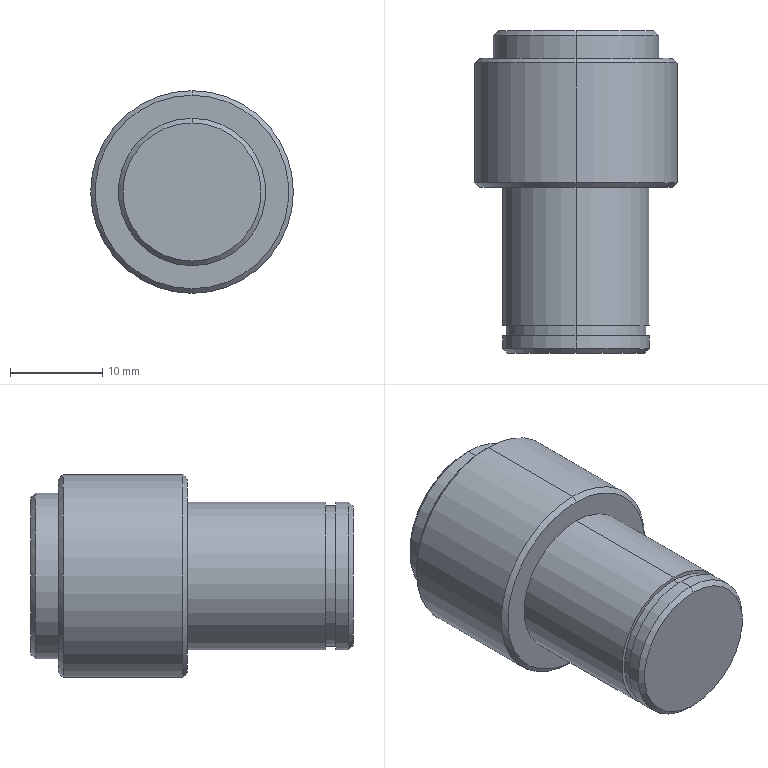Part | STEP file | 02-Support shaft 4 | 1 solid | 24 faces | box 22 x 35 x 22 mm | volume 9653 mm3 | cylinder 10 | cone 8 | plane 6 | commonest cylinder face diameters 16 x4 15.2 x2 18 x2 22 x2
STEP:
#1=CARTESIAN_POINT('',(0.,0.,0.));
#2=DIRECTION('',(0.,0.,1.));
#3=DIRECTION('',(1.,0.,0.));
#4=AXIS2_PLACEMENT_3D('',#1,#2,#3);
#5=CARTESIAN_POINT('',(0.,0.,8.5));
#6=VERTEX_POINT('',#5);
#7=CARTESIAN_POINT('',(0.,0.,-8.5));
#8=VERTEX_POINT('',#7);
#9=CARTESIAN_POINT('',(0.,0.,0.));
#10=DIRECTION('',(0.,1.,0.));
#11=DIRECTION('',(0.,0.,1.));
#12=AXIS2_PLACEMENT_3D('',#9,#10,#11);
#13=CIRCLE('',#12,8.5);
#14=CARTESIAN_POINT('',(0.,0.,0.));
#15=DIRECTION('',(0.,-1.,0.));
#16=DIRECTION('',(0.,0.,-1.));
#17=AXIS2_PLACEMENT_3D('',#14,#15,#16);
#18=CONICAL_SURFACE('',#17,8.5,0.7854);
#19=CARTESIAN_POINT('',(3.142,0.));
#20=DIRECTION('',(-1.,0.));
#21=VECTOR('',#20,1.);
#22=LINE('',#19,#21);
#23=(GEOMETRIC_REPRESENTATION_CONTEXT(2)PARAMETRIC_REPRESENTATION_CONTEXT()REPRESENTATION_CONTEXT('',''));
#24=DEFINITIONAL_REPRESENTATION('',(#22),#23);
#25=PCURVE('',#18,#24);
#26=CARTESIAN_POINT('',(0.,0.,0.));
#27=DIRECTION('',(0.,1.,0.));
#28=DIRECTION('',(0.,0.,1.));
#29=AXIS2_PLACEMENT_3D('',#26,#27,#28);
#30=PLANE('',#29);
#31=CARTESIAN_POINT('',(0.,0.));
#32=DIRECTION('',(1.,0.));
#33=AXIS2_PLACEMENT_2D('',#31,#32);
#34=CIRCLE('',#33,8.5);
#35=(GEOMETRIC_REPRESENTATION_CONTEXT(2)PARAMETRIC_REPRESENTATION_CONTEXT()REPRESENTATION_CONTEXT('',''));
#36=DEFINITIONAL_REPRESENTATION('',(#34),#35);
#37=PCURVE('',#30,#36);
#38=SURFACE_CURVE('',#13,(#25,#37),.PCURVE_S1.);
#39=EDGE_CURVE('',#6,#8,#38,.T.);
#40=ORIENTED_EDGE('',*,*,#39,.F.);
#41=CARTESIAN_POINT('',(0.,-0.5,9.));
#42=VERTEX_POINT('',#41);
#43=CARTESIAN_POINT('',(0.,0.,8.5));
#44=DIRECTION('',(0.,-0.7071,0.7071));
#45=VECTOR('',#44,1.);
#46=LINE('',#43,#45);
#47=CARTESIAN_POINT('',(3.142,0.));
#48=DIRECTION('',(0.,1.));
#49=VECTOR('',#48,1.);
#50=LINE('',#47,#49);
#51=(GEOMETRIC_REPRESENTATION_CONTEXT(2)PARAMETRIC_REPRESENTATION_CONTEXT()REPRESENTATION_CONTEXT('',''));
#52=DEFINITIONAL_REPRESENTATION('',(#50),#51);
#53=PCURVE('',#18,#52);
#54=CARTESIAN_POINT('',(0.,0.,0.));
#55=DIRECTION('',(0.,-1.,0.));
#56=DIRECTION('',(0.,0.,-1.));
#57=AXIS2_PLACEMENT_3D('',#54,#55,#56);
#58=CONICAL_SURFACE('',#57,8.5,0.7854);
#59=CARTESIAN_POINT('',(3.142,0.));
#60=DIRECTION('',(0.,1.));
#61=VECTOR('',#60,1.);
#62=LINE('',#59,#61);
#63=(GEOMETRIC_REPRESENTATION_CONTEXT(2)PARAMETRIC_REPRESENTATION_CONTEXT()REPRESENTATION_CONTEXT('',''));
#64=DEFINITIONAL_REPRESENTATION('',(#62),#63);
#65=PCURVE('',#58,#64);
#66=SURFACE_CURVE('',#46,(#53,#65),.PCURVE_S1.);
#67=EDGE_CURVE('',#6,#42,#66,.T.);
#68=ORIENTED_EDGE('',*,*,#67,.T.);
#69=CARTESIAN_POINT('',(0.,-0.5,-9.));
#70=VERTEX_POINT('',#69);
#71=CARTESIAN_POINT('',(0.,-0.5,0.));
#72=DIRECTION('',(0.,-1.,0.));
#73=DIRECTION('',(0.,0.,1.));
#74=AXIS2_PLACEMENT_3D('',#71,#72,#73);
#75=CIRCLE('',#74,9.);
#76=CARTESIAN_POINT('',(-3.142,0.5));
#77=DIRECTION('',(1.,0.));
#78=VECTOR('',#77,1.);
#79=LINE('',#76,#78);
#80=(GEOMETRIC_REPRESENTATION_CONTEXT(2)PARAMETRIC_REPRESENTATION_CONTEXT()REPRESENTATION_CONTEXT('',''));
#81=DEFINITIONAL_REPRESENTATION('',(#79),#80);
#82=PCURVE('',#18,#81);
#83=CARTESIAN_POINT('',(0.,0.,0.));
#84=DIRECTION('',(0.,1.,0.));
#85=DIRECTION('',(0.,0.,1.));
#86=AXIS2_PLACEMENT_3D('',#83,#84,#85);
#87=CYLINDRICAL_SURFACE('',#86,9.);
#88=CARTESIAN_POINT('',(6.283,-0.5));
#89=DIRECTION('',(-1.,0.));
#90=VECTOR('',#89,1.);
#91=LINE('',#88,#90);
#92=(GEOMETRIC_REPRESENTATION_CONTEXT(2)PARAMETRIC_REPRESENTATION_CONTEXT()REPRESENTATION_CONTEXT('',''));
#93=DEFINITIONAL_REPRESENTATION('',(#91),#92);
#94=PCURVE('',#87,#93);
#95=SURFACE_CURVE('',#75,(#82,#94),.PCURVE_S1.);
#96=EDGE_CURVE('',#70,#42,#95,.T.);
#97=ORIENTED_EDGE('',*,*,#96,.F.);
#98=CARTESIAN_POINT('',(0.,0.,-8.5));
#99=DIRECTION('',(0.,-0.7071,-0.7071));
#100=VECTOR('',#99,1.);
#101=LINE('',#98,#100);
#102=CARTESIAN_POINT('',(0.,0.));
#103=DIRECTION('',(0.,1.));
#104=VECTOR('',#103,1.);
#105=LINE('',#102,#104);
#106=(GEOMETRIC_REPRESENTATION_CONTEXT(2)PARAMETRIC_REPRESENTATION_CONTEXT()REPRESENTATION_CONTEXT('',''));
#107=DEFINITIONAL_REPRESENTATION('',(#105),#106);
#108=PCURVE('',#18,#107);
#109=CARTESIAN_POINT('',(6.283,0.));
#110=DIRECTION('',(0.,1.));
#111=VECTOR('',#110,1.);
#112=LINE('',#109,#111);
#113=(GEOMETRIC_REPRESENTATION_CONTEXT(2)PARAMETRIC_REPRESENTATION_CONTEXT()REPRESENTATION_CONTEXT('',''));
#114=DEFINITIONAL_REPRESENTATION('',(#112),#113);
#115=PCURVE('',#58,#114);
#116=SURFACE_CURVE('',#101,(#108,#115),.PCURVE_S1.);
#117=EDGE_CURVE('',#8,#70,#116,.T.);
#118=ORIENTED_EDGE('',*,*,#117,.F.);
#119=EDGE_LOOP('',(#40,#68,#97,#118));
#120=FACE_BOUND('',#119,.T.);
#121=ADVANCED_FACE('',(#120),#18,.T.);
#122=CARTESIAN_POINT('',(0.,-3.,10.5));
#123=VERTEX_POINT('',#122);
#124=CARTESIAN_POINT('',(0.,-3.,-10.5));
#125=VERTEX_POINT('',#124);
#126=CARTESIAN_POINT('',(0.,-3.,0.));
#127=DIRECTION('',(0.,1.,0.));
#128=DIRECTION('',(0.,0.,1.));
#129=AXIS2_PLACEMENT_3D('',#126,#127,#128);
#130=CIRCLE('',#129,10.5);
#131=CARTESIAN_POINT('',(0.,-3.,0.));
#132=DIRECTION('',(0.,-1.,0.));
#133=DIRECTION('',(0.,0.,-1.));
#134=AXIS2_PLACEMENT_3D('',#131,#132,#133);
#135=CONICAL_SURFACE('',#134,10.5,0.7854);
#136=CARTESIAN_POINT('',(3.142,0.));
#137=DIRECTION('',(-1.,0.));
#138=VECTOR('',#137,1.);
#139=LINE('',#136,#138);
#140=(GEOMETRIC_REPRESENTATION_CONTEXT(2)PARAMETRIC_REPRESENTATION_CONTEXT()REPRESENTATION_CONTEXT('',''));
#141=DEFINITIONAL_REPRESENTATION('',(#139),#140);
#142=PCURVE('',#135,#141);
#143=CARTESIAN_POINT('',(-9.,-3.,0.));
#144=DIRECTION('',(0.,1.,0.));
#145=DIRECTION('',(0.,0.,1.));
#146=AXIS2_PLACEMENT_3D('',#143,#144,#145);
#147=PLANE('',#146);
#148=CARTESIAN_POINT('',(0.,9.));
#149=DIRECTION('',(1.,0.));
#150=AXIS2_PLACEMENT_2D('',#148,#149);
#151=CIRCLE('',#150,10.5);
#152=(GEOMETRIC_REPRESENTATION_CONTEXT(2)PARAMETRIC_REPRESENTATION_CONTEXT()REPRESENTATION_CONTEXT('',''));
#153=DEFINITIONAL_REPRESENTATION('',(#151),#152);
#154=PCURVE('',#147,#153);
#155=SURFACE_CURVE('',#130,(#142,#154),.PCURVE_S1.);
#156=EDGE_CURVE('',#123,#125,#155,.T.);
#157=ORIENTED_EDGE('',*,*,#156,.F.);
#158=CARTESIAN_POINT('',(0.,-3.5,11.));
#159=VERTEX_POINT('',#158);
#160=CARTESIAN_POINT('',(0.,-3.,10.5));
#161=DIRECTION('',(0.,-0.7071,0.7071));
#162=VECTOR('',#161,1.);
#163=LINE('',#160,#162);
#164=CARTESIAN_POINT('',(3.142,0.));
#165=DIRECTION('',(0.,1.));
#166=VECTOR('',#165,1.);
#167=LINE('',#164,#166);
#168=(GEOMETRIC_REPRESENTATION_CONTEXT(2)PARAMETRIC_REPRESENTATION_CONTEXT()REPRESENTATION_CONTEXT('',''));
#169=DEFINITIONAL_REPRESENTATION('',(#167),#168);
#170=PCURVE('',#135,#169);
#171=CARTESIAN_POINT('',(0.,-3.,0.));
#172=DIRECTION('',(0.,-1.,0.));
#173=DIRECTION('',(0.,0.,-1.));
#174=AXIS2_PLACEMENT_3D('',#171,#172,#173);
#175=CONICAL_SURFACE('',#174,10.5,0.7854);
#176=CARTESIAN_POINT('',(3.142,0.));
#177=DIRECTION('',(0.,1.));
#178=VECTOR('',#177,1.);
#179=LINE('',#176,#178);
#180=(GEOMETRIC_REPRESENTATION_CONTEXT(2)PARAMETRIC_REPRESENTATION_CONTEXT()REPRESENTATION_CONTEXT('',''));
#181=DEFINITIONAL_REPRESENTATION('',(#179),#180);
#182=PCURVE('',#175,#181);
#183=SURFACE_CURVE('',#163,(#170,#182),.PCURVE_S1.);
#184=EDGE_CURVE('',#123,#159,#183,.T.);
#185=ORIENTED_EDGE('',*,*,#184,.T.);
#186=CARTESIAN_POINT('',(0.,-3.5,-11.));
#187=VERTEX_POINT('',#186);
#188=CARTESIAN_POINT('',(0.,-3.5,0.));
#189=DIRECTION('',(0.,-1.,0.));
#190=DIRECTION('',(0.,0.,1.));
#191=AXIS2_PLACEMENT_3D('',#188,#189,#190);
#192=CIRCLE('',#191,11.);
#193=CARTESIAN_POINT('',(-3.142,0.5));
#194=DIRECTION('',(1.,0.));
#195=VECTOR('',#194,1.);
#196=LINE('',#193,#195);
#197=(GEOMETRIC_REPRESENTATION_CONTEXT(2)PARAMETRIC_REPRESENTATION_CONTEXT()REPRESENTATION_CONTEXT('',''));
#198=DEFINITIONAL_REPRESENTATION('',(#196),#197);
#199=PCURVE('',#135,#198);
#200=CARTESIAN_POINT('',(0.,0.,0.));
#201=DIRECTION('',(0.,1.,0.));
#202=DIRECTION('',(0.,0.,1.));
#203=AXIS2_PLACEMENT_3D('',#200,#201,#202);
#204=CYLINDRICAL_SURFACE('',#203,11.);
#205=CARTESIAN_POINT('',(6.283,-3.5));
#206=DIRECTION('',(-1.,0.));
#207=VECTOR('',#206,1.);
#208=LINE('',#205,#207);
#209=(GEOMETRIC_REPRESENTATION_CONTEXT(2)PARAMETRIC_REPRESENTATION_CONTEXT()REPRESENTATION_CONTEXT('',''));
#210=DEFINITIONAL_REPRESENTATION('',(#208),#209);
#211=PCURVE('',#204,#210);
#212=SURFACE_CURVE('',#192,(#199,#211),.PCURVE_S1.);
#213=EDGE_CURVE('',#187,#159,#212,.T.);
#214=ORIENTED_EDGE('',*,*,#213,.F.);
#215=CARTESIAN_POINT('',(0.,-3.,-10.5));
#216=DIRECTION('',(0.,-0.7071,-0.7071));
#217=VECTOR('',#216,1.);
#218=LINE('',#215,#217);
#219=CARTESIAN_POINT('',(0.,0.));
#220=DIRECTION('',(0.,1.));
#221=VECTOR('',#220,1.);
#222=LINE('',#219,#221);
#223=(GEOMETRIC_REPRESENTATION_CONTEXT(2)PARAMETRIC_REPRESENTATION_CONTEXT()REPRESENTATION_CONTEXT('',''));
#224=DEFINITIONAL_REPRESENTATION('',(#222),#223);
#225=PCURVE('',#135,#224);
#226=CARTESIAN_POINT('',(6.283,0.));
#227=DIRECTION('',(0.,1.));
#228=VECTOR('',#227,1.);
#229=LINE('',#226,#228);
#230=(GEOMETRIC_REPRESENTATION_CONTEXT(2)PARAMETRIC_REPRESENTATION_CONTEXT()REPRESENTATION_CONTEXT('',''));
#231=DEFINITIONAL_REPRESENTATION('',(#229),#230);
#232=PCURVE('',#175,#231);
#233=SURFACE_CURVE('',#218,(#225,#232),.PCURVE_S1.);
#234=EDGE_CURVE('',#125,#187,#233,.T.);
#235=ORIENTED_EDGE('',*,*,#234,.F.);
#236=EDGE_LOOP('',(#157,#185,#214,#235));
#237=FACE_BOUND('',#236,.T.);
#238=ADVANCED_FACE('',(#237),#135,.T.);
#239=CARTESIAN_POINT('',(0.,-17.,-10.5));
#240=VERTEX_POINT('',#239);
#241=CARTESIAN_POINT('',(0.,-17.,10.5));
#242=VERTEX_POINT('',#241);
#243=CARTESIAN_POINT('',(0.,-17.,0.));
#244=DIRECTION('',(0.,-1.,0.));
#245=DIRECTION('',(0.,0.,-1.));
#246=AXIS2_PLACEMENT_3D('',#243,#244,#245);
#247=CIRCLE('',#246,10.5);
#248=CARTESIAN_POINT('',(0.,-16.5,0.));
#249=DIRECTION('',(0.,1.,0.));
#250=DIRECTION('',(0.,0.,1.));
#251=AXIS2_PLACEMENT_3D('',#248,#249,#250);
#252=CONICAL_SURFACE('',#251,11.,0.7854);
#253=CARTESIAN_POINT('',(3.142,-0.5));
#254=DIRECTION('',(-1.,0.));
#255=VECTOR('',#254,1.);
#256=LINE('',#253,#255);
#257=(GEOMETRIC_REPRESENTATION_CONTEXT(2)PARAMETRIC_REPRESENTATION_CONTEXT()REPRESENTATION_CONTEXT('',''));
#258=DEFINITIONAL_REPRESENTATION('',(#256),#257);
#259=PCURVE('',#252,#258);
#260=CARTESIAN_POINT('',(-11.,-17.,0.));
#261=DIRECTION('',(0.,-1.,0.));
#262=DIRECTION('',(0.,0.,-1.));
#263=AXIS2_PLACEMENT_3D('',#260,#261,#262);
#264=PLANE('',#263);
#265=CARTESIAN_POINT('',(0.,11.));
#266=DIRECTION('',(1.,0.));
#267=AXIS2_PLACEMENT_2D('',#265,#266);
#268=CIRCLE('',#267,10.5);
#269=(GEOMETRIC_REPRESENTATION_CONTEXT(2)PARAMETRIC_REPRESENTATION_CONTEXT()REPRESENTATION_CONTEXT('',''));
#270=DEFINITIONAL_REPRESENTATION('',(#268),#269);
#271=PCURVE('',#264,#270);
#272=SURFACE_CURVE('',#247,(#259,#271),.PCURVE_S1.);
#273=EDGE_CURVE('',#240,#242,#272,.T.);
#274=ORIENTED_EDGE('',*,*,#273,.F.);
#275=CARTESIAN_POINT('',(0.,-16.5,-11.));
#276=VERTEX_POINT('',#275);
#277=CARTESIAN_POINT('',(0.,-16.5,-11.));
#278=DIRECTION('',(0.,0.7071,-0.7071));
#279=VECTOR('',#278,1.);
#280=LINE('',#277,#279);
#281=CARTESIAN_POINT('',(3.142,0.));
#282=DIRECTION('',(0.,1.));
#283=VECTOR('',#282,1.);
#284=LINE('',#281,#283);
#285=(GEOMETRIC_REPRESENTATION_CONTEXT(2)PARAMETRIC_REPRESENTATION_CONTEXT()REPRESENTATION_CONTEXT('',''));
#286=DEFINITIONAL_REPRESENTATION('',(#284),#285);
#287=PCURVE('',#252,#286);
#288=CARTESIAN_POINT('',(0.,-16.5,0.));
#289=DIRECTION('',(0.,1.,0.));
#290=DIRECTION('',(0.,0.,1.));
#291=AXIS2_PLACEMENT_3D('',#288,#289,#290);
#292=CONICAL_SURFACE('',#291,11.,0.7854);
#293=CARTESIAN_POINT('',(3.142,0.));
#294=DIRECTION('',(0.,1.));
#295=VECTOR('',#294,1.);
#296=LINE('',#293,#295);
#297=(GEOMETRIC_REPRESENTATION_CONTEXT(2)PARAMETRIC_REPRESENTATION_CONTEXT()REPRESENTATION_CONTEXT('',''));
#298=DEFINITIONAL_REPRESENTATION('',(#296),#297);
#299=PCURVE('',#292,#298);
#300=SURFACE_CURVE('',#280,(#287,#299),.PCURVE_S1.);
#301=EDGE_CURVE('',#240,#276,#300,.T.);
#302=ORIENTED_EDGE('',*,*,#301,.T.);
#303=CARTESIAN_POINT('',(0.,-16.5,11.));
#304=VERTEX_POINT('',#303);
#305=CARTESIAN_POINT('',(0.,-16.5,0.));
#306=DIRECTION('',(0.,1.,0.));
#307=DIRECTION('',(0.,0.,-1.));
#308=AXIS2_PLACEMENT_3D('',#305,#306,#307);
#309=CIRCLE('',#308,11.);
#310=CARTESIAN_POINT('',(-3.142,0.));
#311=DIRECTION('',(1.,0.));
#312=VECTOR('',#311,1.);
#313=LINE('',#310,#312);
#314=(GEOMETRIC_REPRESENTATION_CONTEXT(2)PARAMETRIC_REPRESENTATION_CONTEXT()REPRESENTATION_CONTEXT('',''));
#315=DEFINITIONAL_REPRESENTATION('',(#313),#314);
#316=PCURVE('',#252,#315);
#317=CARTESIAN_POINT('',(-3.142,-16.5));
#318=DIRECTION('',(1.,0.));
#319=VECTOR('',#318,1.);
#320=LINE('',#317,#319);
#321=(GEOMETRIC_REPRESENTATION_CONTEXT(2)PARAMETRIC_REPRESENTATION_CONTEXT()REPRESENTATION_CONTEXT('',''));
#322=DEFINITIONAL_REPRESENTATION('',(#320),#321);
#323=PCURVE('',#204,#322);
#324=SURFACE_CURVE('',#309,(#316,#323),.PCURVE_S1.);
#325=EDGE_CURVE('',#304,#276,#324,.T.);
#326=ORIENTED_EDGE('',*,*,#325,.F.);
#327=CARTESIAN_POINT('',(0.,-16.5,11.));
#328=DIRECTION('',(0.,0.7071,0.7071));
#329=VECTOR('',#328,1.);
#330=LINE('',#327,#329);
#331=CARTESIAN_POINT('',(0.,0.));
#332=DIRECTION('',(0.,1.));
#333=VECTOR('',#332,1.);
#334=LINE('',#331,#333);
#335=(GEOMETRIC_REPRESENTATION_CONTEXT(2)PARAMETRIC_REPRESENTATION_CONTEXT()REPRESENTATION_CONTEXT('',''));
#336=DEFINITIONAL_REPRESENTATION('',(#334),#335);
#337=PCURVE('',#252,#336);
#338=CARTESIAN_POINT('',(6.283,0.));
#339=DIRECTION('',(0.,1.));
#340=VECTOR('',#339,1.);
#341=LINE('',#338,#340);
#342=(GEOMETRIC_REPRESENTATION_CONTEXT(2)PARAMETRIC_REPRESENTATION_CONTEXT()REPRESENTATION_CONTEXT('',''));
#343=DEFINITIONAL_REPRESENTATION('',(#341),#342);
#344=PCURVE('',#292,#343);
#345=SURFACE_CURVE('',#330,(#337,#344),.PCURVE_S1.);
#346=EDGE_CURVE('',#242,#304,#345,.T.);
#347=ORIENTED_EDGE('',*,*,#346,.F.);
#348=EDGE_LOOP('',(#274,#302,#326,#347));
#349=FACE_BOUND('',#348,.T.);
#350=ADVANCED_FACE('',(#349),#252,.T.);
#351=CARTESIAN_POINT('',(0.,-35.,-7.5));
#352=VERTEX_POINT('',#351);
#353=CARTESIAN_POINT('',(0.,-35.,7.5));
#354=VERTEX_POINT('',#353);
#355=CARTESIAN_POINT('',(0.,-35.,0.));
#356=DIRECTION('',(0.,-1.,0.));
#357=DIRECTION('',(0.,0.,-1.));
#358=AXIS2_PLACEMENT_3D('',#355,#356,#357);
#359=CIRCLE('',#358,7.5);
#360=CARTESIAN_POINT('',(0.,-34.5,0.));
#361=DIRECTION('',(0.,1.,0.));
#362=DIRECTION('',(0.,0.,1.));
#363=AXIS2_PLACEMENT_3D('',#360,#361,#362);
#364=CONICAL_SURFACE('',#363,8.,0.7854);
#365=CARTESIAN_POINT('',(3.142,-0.5));
#366=DIRECTION('',(-1.,0.));
#367=VECTOR('',#366,1.);
#368=LINE('',#365,#367);
#369=(GEOMETRIC_REPRESENTATION_CONTEXT(2)PARAMETRIC_REPRESENTATION_CONTEXT()REPRESENTATION_CONTEXT('',''));
#370=DEFINITIONAL_REPRESENTATION('',(#368),#369);
#371=PCURVE('',#364,#370);
#372=CARTESIAN_POINT('',(-8.,-35.,0.));
#373=DIRECTION('',(0.,-1.,0.));
#374=DIRECTION('',(0.,0.,-1.));
#375=AXIS2_PLACEMENT_3D('',#372,#373,#374);
#376=PLANE('',#375);
#377=CARTESIAN_POINT('',(0.,8.));
#378=DIRECTION('',(1.,0.));
#379=AXIS2_PLACEMENT_2D('',#377,#378);
#380=CIRCLE('',#379,7.5);
#381=(GEOMETRIC_REPRESENTATION_CONTEXT(2)PARAMETRIC_REPRESENTATION_CONTEXT()REPRESENTATION_CONTEXT('',''));
#382=DEFINITIONAL_REPRESENTATION('',(#380),#381);
#383=PCURVE('',#376,#382);
#384=SURFACE_CURVE('',#359,(#371,#383),.PCURVE_S1.);
#385=EDGE_CURVE('',#352,#354,#384,.T.);
#386=ORIENTED_EDGE('',*,*,#385,.F.);
#387=CARTESIAN_POINT('',(0.,-34.5,-8.));
#388=VERTEX_POINT('',#387);
#389=CARTESIAN_POINT('',(0.,-34.5,-8.));
#390=DIRECTION('',(0.,0.7071,-0.7071));
#391=VECTOR('',#390,1.);
#392=LINE('',#389,#391);
#393=CARTESIAN_POINT('',(3.142,0.));
#394=DIRECTION('',(0.,1.));
#395=VECTOR('',#394,1.);
#396=LINE('',#393,#395);
#397=(GEOMETRIC_REPRESENTATION_CONTEXT(2)PARAMETRIC_REPRESENTATION_CONTEXT()REPRESENTATION_CONTEXT('',''));
#398=DEFINITIONAL_REPRESENTATION('',(#396),#397);
#399=PCURVE('',#364,#398);
#400=CARTESIAN_POINT('',(0.,-34.5,0.));
#401=DIRECTION('',(0.,1.,0.));
#402=DIRECTION('',(0.,0.,1.));
#403=AXIS2_PLACEMENT_3D('',#400,#401,#402);
#404=CONICAL_SURFACE('',#403,8.,0.7854);
#405=CARTESIAN_POINT('',(3.142,0.));
#406=DIRECTION('',(0.,1.));
#407=VECTOR('',#406,1.);
#408=LINE('',#405,#407);
#409=(GEOMETRIC_REPRESENTATION_CONTEXT(2)PARAMETRIC_REPRESENTATION_CONTEXT()REPRESENTATION_CONTEXT('',''));
#410=DEFINITIONAL_REPRESENTATION('',(#408),#409);
#411=PCURVE('',#404,#410);
#412=SURFACE_CURVE('',#392,(#399,#411),.PCURVE_S1.);
#413=EDGE_CURVE('',#352,#388,#412,.T.);
#414=ORIENTED_EDGE('',*,*,#413,.T.);
#415=CARTESIAN_POINT('',(0.,-34.5,8.));
#416=VERTEX_POINT('',#415);
#417=CARTESIAN_POINT('',(0.,-34.5,0.));
#418=DIRECTION('',(0.,1.,0.));
#419=DIRECTION('',(0.,0.,-1.));
#420=AXIS2_PLACEMENT_3D('',#417,#418,#419);
#421=CIRCLE('',#420,8.);
#422=CARTESIAN_POINT('',(-3.142,0.));
#423=DIRECTION('',(1.,0.));
#424=VECTOR('',#423,1.);
#425=LINE('',#422,#424);
#426=(GEOMETRIC_REPRESENTATION_CONTEXT(2)PARAMETRIC_REPRESENTATION_CONTEXT()REPRESENTATION_CONTEXT('',''));
#427=DEFINITIONAL_REPRESENTATION('',(#425),#426);
#428=PCURVE('',#364,#427);
#429=CARTESIAN_POINT('',(0.,0.,0.));
#430=DIRECTION('',(0.,1.,0.));
#431=DIRECTION('',(0.,0.,1.));
#432=AXIS2_PLACEMENT_3D('',#429,#430,#431);
#433=CYLINDRICAL_SURFACE('',#432,8.);
#434=CARTESIAN_POINT('',(-3.142,-34.5));
#435=DIRECTION('',(1.,0.));
#436=VECTOR('',#435,1.);
#437=LINE('',#434,#436);
#438=(GEOMETRIC_REPRESENTATION_CONTEXT(2)PARAMETRIC_REPRESENTATION_CONTEXT()REPRESENTATION_CONTEXT('',''));
#439=DEFINITIONAL_REPRESENTATION('',(#437),#438);
#440=PCURVE('',#433,#439);
#441=SURFACE_CURVE('',#421,(#428,#440),.PCURVE_S1.);
#442=EDGE_CURVE('',#416,#388,#441,.T.);
#443=ORIENTED_EDGE('',*,*,#442,.F.);
#444=CARTESIAN_POINT('',(0.,-34.5,8.));
#445=DIRECTION('',(0.,0.7071,0.7071));
#446=VECTOR('',#445,1.);
#447=LINE('',#444,#446);
#448=CARTESIAN_POINT('',(0.,0.));
#449=DIRECTION('',(0.,1.));
#450=VECTOR('',#449,1.);
#451=LINE('',#448,#450);
#452=(GEOMETRIC_REPRESENTATION_CONTEXT(2)PARAMETRIC_REPRESENTATION_CONTEXT()REPRESENTATION_CONTEXT('',''));
#453=DEFINITIONAL_REPRESENTATION('',(#451),#452);
#454=PCURVE('',#364,#453);
#455=CARTESIAN_POINT('',(6.283,0.));
#456=DIRECTION('',(0.,1.));
#457=VECTOR('',#456,1.);
#458=LINE('',#455,#457);
#459=(GEOMETRIC_REPRESENTATION_CONTEXT(2)PARAMETRIC_REPRESENTATION_CONTEXT()REPRESENTATION_CONTEXT('',''));
#460=DEFINITIONAL_REPRESENTATION('',(#458),#459);
#461=PCURVE('',#404,#460);
#462=SURFACE_CURVE('',#447,(#454,#461),.PCURVE_S1.);
#463=EDGE_CURVE('',#354,#416,#462,.T.);
#464=ORIENTED_EDGE('',*,*,#463,.F.);
#465=EDGE_LOOP('',(#386,#414,#443,#464));
#466=FACE_BOUND('',#465,.T.);
#467=ADVANCED_FACE('',(#466),#364,.T.);
#468=ORIENTED_EDGE('',*,*,#442,.T.);
#469=CARTESIAN_POINT('',(0.,-33.1,-8.));
#470=VERTEX_POINT('',#469);
#471=CARTESIAN_POINT('',(0.,0.,-8.));
#472=DIRECTION('',(0.,1.,0.));
#473=VECTOR('',#472,1.);
#474=LINE('',#471,#473);
#475=CARTESIAN_POINT('',(3.142,0.));
#476=DIRECTION('',(0.,1.));
#477=VECTOR('',#476,1.);
#478=LINE('',#475,#477);
#479=(GEOMETRIC_REPRESENTATION_CONTEXT(2)PARAMETRIC_REPRESENTATION_CONTEXT()REPRESENTATION_CONTEXT('',''));
#480=DEFINITIONAL_REPRESENTATION('',(#478),#479);
#481=PCURVE('',#433,#480);
#482=CARTESIAN_POINT('',(0.,0.,0.));
#483=DIRECTION('',(0.,1.,0.));
#484=DIRECTION('',(0.,0.,1.));
#485=AXIS2_PLACEMENT_3D('',#482,#483,#484);
#486=CYLINDRICAL_SURFACE('',#485,8.);
#487=CARTESIAN_POINT('',(3.142,0.));
#488=DIRECTION('',(0.,1.));
#489=VECTOR('',#488,1.);
#490=LINE('',#487,#489);
#491=(GEOMETRIC_REPRESENTATION_CONTEXT(2)PARAMETRIC_REPRESENTATION_CONTEXT()REPRESENTATION_CONTEXT('',''));
#492=DEFINITIONAL_REPRESENTATION('',(#490),#491);
#493=PCURVE('',#486,#492);
#494=SURFACE_CURVE('',#474,(#481,#493),.PCURVE_S1.);
#495=EDGE_CURVE('',#388,#470,#494,.T.);
#496=ORIENTED_EDGE('',*,*,#495,.T.);
#497=CARTESIAN_POINT('',(0.,-33.1,8.));
#498=VERTEX_POINT('',#497);
#499=CARTESIAN_POINT('',(0.,-33.1,0.));
#500=DIRECTION('',(0.,1.,0.));
#501=DIRECTION('',(0.,0.,1.));
#502=AXIS2_PLACEMENT_3D('',#499,#500,#501);
#503=CIRCLE('',#502,8.);
#504=CARTESIAN_POINT('',(0.,-33.1));
#505=DIRECTION('',(1.,0.));
#506=VECTOR('',#505,1.);
#507=LINE('',#504,#506);
#508=(GEOMETRIC_REPRESENTATION_CONTEXT(2)PARAMETRIC_REPRESENTATION_CONTEXT()REPRESENTATION_CONTEXT('',''));
#509=DEFINITIONAL_REPRESENTATION('',(#507),#508);
#510=PCURVE('',#433,#509);
#511=CARTESIAN_POINT('',(-7.6,-33.1,0.));
#512=DIRECTION('',(0.,1.,0.));
#513=DIRECTION('',(0.,0.,1.));
#514=AXIS2_PLACEMENT_3D('',#511,#512,#513);
#515=PLANE('',#514);
#516=CARTESIAN_POINT('',(0.,7.6));
#517=DIRECTION('',(1.,0.));
#518=AXIS2_PLACEMENT_2D('',#516,#517);
#519=CIRCLE('',#518,8.);
#520=(GEOMETRIC_REPRESENTATION_CONTEXT(2)PARAMETRIC_REPRESENTATION_CONTEXT()REPRESENTATION_CONTEXT('',''));
#521=DEFINITIONAL_REPRESENTATION('',(#519),#520);
#522=PCURVE('',#515,#521);
#523=SURFACE_CURVE('',#503,(#510,#522),.PCURVE_S1.);
#524=EDGE_CURVE('',#498,#470,#523,.T.);
#525=ORIENTED_EDGE('',*,*,#524,.F.);
#526=CARTESIAN_POINT('',(0.,0.,8.));
#527=DIRECTION('',(0.,1.,0.));
#528=VECTOR('',#527,1.);
#529=LINE('',#526,#528);
#530=CARTESIAN_POINT('',(0.,0.));
#531=DIRECTION('',(0.,1.));
#532=VECTOR('',#531,1.);
#533=LINE('',#530,#532);
#534=(GEOMETRIC_REPRESENTATION_CONTEXT(2)PARAMETRIC_REPRESENTATION_CONTEXT()REPRESENTATION_CONTEXT('',''));
#535=DEFINITIONAL_REPRESENTATION('',(#533),#534);
#536=PCURVE('',#433,#535);
#537=CARTESIAN_POINT('',(6.283,0.));
#538=DIRECTION('',(0.,1.));
#539=VECTOR('',#538,1.);
#540=LINE('',#537,#539);
#541=(GEOMETRIC_REPRESENTATION_CONTEXT(2)PARAMETRIC_REPRESENTATION_CONTEXT()REPRESENTATION_CONTEXT('',''));
#542=DEFINITIONAL_REPRESENTATION('',(#540),#541);
#543=PCURVE('',#486,#542);
#544=SURFACE_CURVE('',#529,(#536,#543),.PCURVE_S1.);
#545=EDGE_CURVE('',#416,#498,#544,.T.);
#546=ORIENTED_EDGE('',*,*,#545,.F.);
#547=EDGE_LOOP('',(#468,#496,#525,#546));
#548=FACE_BOUND('',#547,.T.);
#549=ADVANCED_FACE('',(#548),#433,.T.);
#550=CARTESIAN_POINT('',(0.,-33.1,7.6));
#551=VERTEX_POINT('',#550);
#552=CARTESIAN_POINT('',(0.,-33.1,-7.6));
#553=VERTEX_POINT('',#552);
#554=CARTESIAN_POINT('',(0.,-33.1,0.));
#555=DIRECTION('',(0.,1.,0.));
#556=DIRECTION('',(0.,0.,1.));
#557=AXIS2_PLACEMENT_3D('',#554,#555,#556);
#558=CIRCLE('',#557,7.6);
#559=CARTESIAN_POINT('',(0.,0.,0.));
#560=DIRECTION('',(0.,1.,0.));
#561=DIRECTION('',(0.,0.,1.));
#562=AXIS2_PLACEMENT_3D('',#559,#560,#561);
#563=CYLINDRICAL_SURFACE('',#562,7.6);
#564=CARTESIAN_POINT('',(0.,-33.1));
#565=DIRECTION('',(1.,0.));
#566=VECTOR('',#565,1.);
#567=LINE('',#564,#566);
#568=(GEOMETRIC_REPRESENTATION_CONTEXT(2)PARAMETRIC_REPRESENTATION_CONTEXT()REPRESENTATION_CONTEXT('',''));
#569=DEFINITIONAL_REPRESENTATION('',(#567),#568);
#570=PCURVE('',#563,#569);
#571=CARTESIAN_POINT('',(0.,7.6));
#572=DIRECTION('',(1.,0.));
#573=AXIS2_PLACEMENT_2D('',#571,#572);
#574=CIRCLE('',#573,7.6);
#575=(GEOMETRIC_REPRESENTATION_CONTEXT(2)PARAMETRIC_REPRESENTATION_CONTEXT()REPRESENTATION_CONTEXT('',''));
#576=DEFINITIONAL_REPRESENTATION('',(#574),#575);
#577=PCURVE('',#515,#576);
#578=SURFACE_CURVE('',#558,(#570,#577),.PCURVE_S1.);
#579=EDGE_CURVE('',#551,#553,#578,.T.);
#580=ORIENTED_EDGE('',*,*,#579,.T.);
#581=CARTESIAN_POINT('',(0.,-32.,-7.6));
#582=VERTEX_POINT('',#581);
#583=CARTESIAN_POINT('',(0.,0.,-7.6));
#584=DIRECTION('',(0.,1.,0.));
#585=VECTOR('',#584,1.);
#586=LINE('',#583,#585);
#587=CARTESIAN_POINT('',(3.142,0.));
#588=DIRECTION('',(0.,1.));
#589=VECTOR('',#588,1.);
#590=LINE('',#587,#589);
#591=(GEOMETRIC_REPRESENTATION_CONTEXT(2)PARAMETRIC_REPRESENTATION_CONTEXT()REPRESENTATION_CONTEXT('',''));
#592=DEFINITIONAL_REPRESENTATION('',(#590),#591);
#593=PCURVE('',#563,#592);
#594=CARTESIAN_POINT('',(0.,0.,0.));
#595=DIRECTION('',(0.,1.,0.));
#596=DIRECTION('',(0.,0.,1.));
#597=AXIS2_PLACEMENT_3D('',#594,#595,#596);
#598=CYLINDRICAL_SURFACE('',#597,7.6);
#599=CARTESIAN_POINT('',(3.142,0.));
#600=DIRECTION('',(0.,1.));
#601=VECTOR('',#600,1.);
#602=LINE('',#599,#601);
#603=(GEOMETRIC_REPRESENTATION_CONTEXT(2)PARAMETRIC_REPRESENTATION_CONTEXT()REPRESENTATION_CONTEXT('',''));
#604=DEFINITIONAL_REPRESENTATION('',(#602),#603);
#605=PCURVE('',#598,#604);
#606=SURFACE_CURVE('',#586,(#593,#605),.PCURVE_S1.);
#607=EDGE_CURVE('',#553,#582,#606,.T.);
#608=ORIENTED_EDGE('',*,*,#607,.T.);
#609=CARTESIAN_POINT('',(0.,-32.,7.6));
#610=VERTEX_POINT('',#609);
#611=CARTESIAN_POINT('',(0.,-32.,0.));
#612=DIRECTION('',(0.,1.,0.));
#613=DIRECTION('',(0.,0.,1.));
#614=AXIS2_PLACEMENT_3D('',#611,#612,#613);
#615=CIRCLE('',#614,7.6);
#616=CARTESIAN_POINT('',(0.,-32.));
#617=DIRECTION('',(1.,0.));
#618=VECTOR('',#617,1.);
#619=LINE('',#616,#618);
#620=(GEOMETRIC_REPRESENTATION_CONTEXT(2)PARAMETRIC_REPRESENTATION_CONTEXT()REPRESENTATION_CONTEXT('',''));
#621=DEFINITIONAL_REPRESENTATION('',(#619),#620);
#622=PCURVE('',#563,#621);
#623=CARTESIAN_POINT('',(-8.,-32.,0.));
#624=DIRECTION('',(0.,-1.,0.));
#625=DIRECTION('',(0.,0.,-1.));
#626=AXIS2_PLACEMENT_3D('',#623,#624,#625);
#627=PLANE('',#626);
#628=CARTESIAN_POINT('',(-7.6,8.));
#629=CARTESIAN_POINT('',(-7.6,21.164));
#630=CARTESIAN_POINT('',(3.8,14.582));
#631=CARTESIAN_POINT('',(15.2,8.));
#632=CARTESIAN_POINT('',(3.8,1.418));
#633=CARTESIAN_POINT('',(-7.6,-5.164));
#634=CARTESIAN_POINT('',(-7.6,8.));
#635=(BOUNDED_CURVE()B_SPLINE_CURVE(2,(#628,#629,#630,#631,#632,#633,#634),.UNSPECIFIED.,.T.,.F.)B_SPLINE_CURVE_WITH_KNOTS((1,2,2,2,2,1),(-2.094,0.,2.094,4.189,6.283,8.378),.UNSPECIFIED.)CURVE()GEOMETRIC_REPRESENTATION_ITEM()RATIONAL_B_SPLINE_CURVE((1.,0.5,1.,0.5,1.,0.5,1.))REPRESENTATION_ITEM(''));
#636=(GEOMETRIC_REPRESENTATION_CONTEXT(2)PARAMETRIC_REPRESENTATION_CONTEXT()REPRESENTATION_CONTEXT('',''));
#637=DEFINITIONAL_REPRESENTATION('',(#635),#636);
#638=PCURVE('',#627,#637);
#639=SURFACE_CURVE('',#615,(#622,#638),.PCURVE_S1.);
#640=EDGE_CURVE('',#610,#582,#639,.T.);
#641=ORIENTED_EDGE('',*,*,#640,.F.);
#642=CARTESIAN_POINT('',(0.,0.,7.6));
#643=DIRECTION('',(0.,1.,0.));
#644=VECTOR('',#643,1.);
#645=LINE('',#642,#644);
#646=CARTESIAN_POINT('',(0.,0.));
#647=DIRECTION('',(0.,1.));
#648=VECTOR('',#647,1.);
#649=LINE('',#646,#648);
#650=(GEOMETRIC_REPRESENTATION_CONTEXT(2)PARAMETRIC_REPRESENTATION_CONTEXT()REPRESENTATION_CONTEXT('',''));
#651=DEFINITIONAL_REPRESENTATION('',(#649),#650);
#652=PCURVE('',#563,#651);
#653=CARTESIAN_POINT('',(6.283,0.));
#654=DIRECTION('',(0.,1.));
#655=VECTOR('',#654,1.);
#656=LINE('',#653,#655);
#657=(GEOMETRIC_REPRESENTATION_CONTEXT(2)PARAMETRIC_REPRESENTATION_CONTEXT()REPRESENTATION_CONTEXT('',''));
#658=DEFINITIONAL_REPRESENTATION('',(#656),#657);
#659=PCURVE('',#598,#658);
#660=SURFACE_CURVE('',#645,(#652,#659),.PCURVE_S1.);
#661=EDGE_CURVE('',#551,#610,#660,.T.);
#662=ORIENTED_EDGE('',*,*,#661,.F.);
#663=EDGE_LOOP('',(#580,#608,#641,#662));
#664=FACE_BOUND('',#663,.T.);
#665=ADVANCED_FACE('',(#664),#563,.T.);
#666=CARTESIAN_POINT('',(0.,-32.,8.));
#667=VERTEX_POINT('',#666);
#668=CARTESIAN_POINT('',(0.,-32.,-8.));
#669=VERTEX_POINT('',#668);
#670=CARTESIAN_POINT('',(0.,-32.,0.));
#671=DIRECTION('',(0.,1.,0.));
#672=DIRECTION('',(0.,0.,1.));
#673=AXIS2_PLACEMENT_3D('',#670,#671,#672);
#674=CIRCLE('',#673,8.);
#675=CARTESIAN_POINT('',(0.,0.,0.));
#676=DIRECTION('',(0.,1.,0.));
#677=DIRECTION('',(0.,0.,1.));
#678=AXIS2_PLACEMENT_3D('',#675,#676,#677);
#679=CYLINDRICAL_SURFACE('',#678,8.);
#680=CARTESIAN_POINT('',(0.,-32.));
#681=DIRECTION('',(1.,0.));
#682=VECTOR('',#681,1.);
#683=LINE('',#680,#682);
#684=(GEOMETRIC_REPRESENTATION_CONTEXT(2)PARAMETRIC_REPRESENTATION_CONTEXT()REPRESENTATION_CONTEXT('',''));
#685=DEFINITIONAL_REPRESENTATION('',(#683),#684);
#686=PCURVE('',#679,#685);
#687=CARTESIAN_POINT('',(-8.,8.));
#688=CARTESIAN_POINT('',(-8.,21.856));
#689=CARTESIAN_POINT('',(4.,14.928));
#690=CARTESIAN_POINT('',(16.,8.));
#691=CARTESIAN_POINT('',(4.,1.072));
#692=CARTESIAN_POINT('',(-8.,-5.856));
#693=CARTESIAN_POINT('',(-8.,8.));
#694=(BOUNDED_CURVE()B_SPLINE_CURVE(2,(#687,#688,#689,#690,#691,#692,#693),.UNSPECIFIED.,.T.,.F.)B_SPLINE_CURVE_WITH_KNOTS((1,2,2,2,2,1),(-2.094,0.,2.094,4.189,6.283,8.378),.UNSPECIFIED.)CURVE()GEOMETRIC_REPRESENTATION_ITEM()RATIONAL_B_SPLINE_CURVE((1.,0.5,1.,0.5,1.,0.5,1.))REPRESENTATION_ITEM(''));
#695=(GEOMETRIC_REPRESENTATION_CONTEXT(2)PARAMETRIC_REPRESENTATION_CONTEXT()REPRESENTATION_CONTEXT('',''));
#696=DEFINITIONAL_REPRESENTATION('',(#694),#695);
#697=PCURVE('',#627,#696);
#698=SURFACE_CURVE('',#674,(#686,#697),.PCURVE_S1.);
#699=EDGE_CURVE('',#667,#669,#698,.T.);
#700=ORIENTED_EDGE('',*,*,#699,.T.);
#701=CARTESIAN_POINT('',(0.,-17.,-8.));
#702=VERTEX_POINT('',#701);
#703=CARTESIAN_POINT('',(0.,0.,-8.));
#704=DIRECTION('',(0.,1.,0.));
#705=VECTOR('',#704,1.);
#706=LINE('',#703,#705);
#707=CARTESIAN_POINT('',(3.142,0.));
#708=DIRECTION('',(0.,1.));
#709=VECTOR('',#708,1.);
#710=LINE('',#707,#709);
#711=(GEOMETRIC_REPRESENTATION_CONTEXT(2)PARAMETRIC_REPRESENTATION_CONTEXT()REPRESENTATION_CONTEXT('',''));
#712=DEFINITIONAL_REPRESENTATION('',(#710),#711);
#713=PCURVE('',#679,#712);
#714=CARTESIAN_POINT('',(0.,0.,0.));
#715=DIRECTION('',(0.,1.,0.));
#716=DIRECTION('',(0.,0.,1.));
#717=AXIS2_PLACEMENT_3D('',#714,#715,#716);
#718=CYLINDRICAL_SURFACE('',#717,8.);
#719=CARTESIAN_POINT('',(3.142,0.));
#720=DIRECTION('',(0.,1.));
#721=VECTOR('',#720,1.);
#722=LINE('',#719,#721);
#723=(GEOMETRIC_REPRESENTATION_CONTEXT(2)PARAMETRIC_REPRESENTATION_CONTEXT()REPRESENTATION_CONTEXT('',''));
#724=DEFINITIONAL_REPRESENTATION('',(#722),#723);
#725=PCURVE('',#718,#724);
#726=SURFACE_CURVE('',#706,(#713,#725),.PCURVE_S1.);
#727=EDGE_CURVE('',#669,#702,#726,.T.);
#728=ORIENTED_EDGE('',*,*,#727,.T.);
#729=CARTESIAN_POINT('',(0.,-17.,8.));
#730=VERTEX_POINT('',#729);
#731=CARTESIAN_POINT('',(0.,-17.,0.));
#732=DIRECTION('',(0.,1.,0.));
#733=DIRECTION('',(0.,0.,1.));
#734=AXIS2_PLACEMENT_3D('',#731,#732,#733);
#735=CIRCLE('',#734,8.);
#736=CARTESIAN_POINT('',(0.,-17.));
#737=DIRECTION('',(1.,0.));
#738=VECTOR('',#737,1.);
#739=LINE('',#736,#738);
#740=(GEOMETRIC_REPRESENTATION_CONTEXT(2)PARAMETRIC_REPRESENTATION_CONTEXT()REPRESENTATION_CONTEXT('',''));
#741=DEFINITIONAL_REPRESENTATION('',(#739),#740);
#742=PCURVE('',#679,#741);
#743=CARTESIAN_POINT('',(-8.,11.));
#744=CARTESIAN_POINT('',(-8.,24.856));
#745=CARTESIAN_POINT('',(4.,17.928));
#746=CARTESIAN_POINT('',(16.,11.));
#747=CARTESIAN_POINT('',(4.,4.072));
#748=CARTESIAN_POINT('',(-8.,-2.856));
#749=CARTESIAN_POINT('',(-8.,11.));
#750=(BOUNDED_CURVE()B_SPLINE_CURVE(2,(#743,#744,#745,#746,#747,#748,#749),.UNSPECIFIED.,.T.,.F.)B_SPLINE_CURVE_WITH_KNOTS((1,2,2,2,2,1),(-2.094,0.,2.094,4.189,6.283,8.378),.UNSPECIFIED.)CURVE()GEOMETRIC_REPRESENTATION_ITEM()RATIONAL_B_SPLINE_CURVE((1.,0.5,1.,0.5,1.,0.5,1.))REPRESENTATION_ITEM(''));
#751=(GEOMETRIC_REPRESENTATION_CONTEXT(2)PARAMETRIC_REPRESENTATION_CONTEXT()REPRESENTATION_CONTEXT('',''));
#752=DEFINITIONAL_REPRESENTATION('',(#750),#751);
#753=PCURVE('',#264,#752);
#754=SURFACE_CURVE('',#735,(#742,#753),.PCURVE_S1.);
#755=EDGE_CURVE('',#730,#702,#754,.T.);
#756=ORIENTED_EDGE('',*,*,#755,.F.);
#757=CARTESIAN_POINT('',(0.,0.,8.));
#758=DIRECTION('',(0.,1.,0.));
#759=VECTOR('',#758,1.);
#760=LINE('',#757,#759);
#761=CARTESIAN_POINT('',(0.,0.));
#762=DIRECTION('',(0.,1.));
#763=VECTOR('',#762,1.);
#764=LINE('',#761,#763);
#765=(GEOMETRIC_REPRESENTATION_CONTEXT(2)PARAMETRIC_REPRESENTATION_CONTEXT()REPRESENTATION_CONTEXT('',''));
#766=DEFINITIONAL_REPRESENTATION('',(#764),#765);
#767=PCURVE('',#679,#766);
#768=CARTESIAN_POINT('',(6.283,0.));
#769=DIRECTION('',(0.,1.));
#770=VECTOR('',#769,1.);
#771=LINE('',#768,#770);
#772=(GEOMETRIC_REPRESENTATION_CONTEXT(2)PARAMETRIC_REPRESENTATION_CONTEXT()REPRESENTATION_CONTEXT('',''));
#773=DEFINITIONAL_REPRESENTATION('',(#771),#772);
#774=PCURVE('',#718,#773);
#775=SURFACE_CURVE('',#760,(#767,#774),.PCURVE_S1.);
#776=EDGE_CURVE('',#667,#730,#775,.T.);
#777=ORIENTED_EDGE('',*,*,#776,.F.);
#778=EDGE_LOOP('',(#700,#728,#756,#777));
#779=FACE_BOUND('',#778,.T.);
#780=ADVANCED_FACE('',(#779),#679,.T.);
#781=ORIENTED_EDGE('',*,*,#325,.T.);
#782=CARTESIAN_POINT('',(0.,0.,-11.));
#783=DIRECTION('',(0.,1.,0.));
#784=VECTOR('',#783,1.);
#785=LINE('',#782,#784);
#786=CARTESIAN_POINT('',(3.142,0.));
#787=DIRECTION('',(0.,1.));
#788=VECTOR('',#787,1.);
#789=LINE('',#786,#788);
#790=(GEOMETRIC_REPRESENTATION_CONTEXT(2)PARAMETRIC_REPRESENTATION_CONTEXT()REPRESENTATION_CONTEXT('',''));
#791=DEFINITIONAL_REPRESENTATION('',(#789),#790);
#792=PCURVE('',#204,#791);
#793=CARTESIAN_POINT('',(0.,0.,0.));
#794=DIRECTION('',(0.,1.,0.));
#795=DIRECTION('',(0.,0.,1.));
#796=AXIS2_PLACEMENT_3D('',#793,#794,#795);
#797=CYLINDRICAL_SURFACE('',#796,11.);
#798=CARTESIAN_POINT('',(3.142,0.));
#799=DIRECTION('',(0.,1.));
#800=VECTOR('',#799,1.);
#801=LINE('',#798,#800);
#802=(GEOMETRIC_REPRESENTATION_CONTEXT(2)PARAMETRIC_REPRESENTATION_CONTEXT()REPRESENTATION_CONTEXT('',''));
#803=DEFINITIONAL_REPRESENTATION('',(#801),#802);
#804=PCURVE('',#797,#803);
#805=SURFACE_CURVE('',#785,(#792,#804),.PCURVE_S1.);
#806=EDGE_CURVE('',#276,#187,#805,.T.);
#807=ORIENTED_EDGE('',*,*,#806,.T.);
#808=ORIENTED_EDGE('',*,*,#213,.T.);
#809=CARTESIAN_POINT('',(0.,0.,11.));
#810=DIRECTION('',(0.,1.,0.));
#811=VECTOR('',#810,1.);
#812=LINE('',#809,#811);
#813=CARTESIAN_POINT('',(0.,0.));
#814=DIRECTION('',(0.,1.));
#815=VECTOR('',#814,1.);
#816=LINE('',#813,#815);
#817=(GEOMETRIC_REPRESENTATION_CONTEXT(2)PARAMETRIC_REPRESENTATION_CONTEXT()REPRESENTATION_CONTEXT('',''));
#818=DEFINITIONAL_REPRESENTATION('',(#816),#817);
#819=PCURVE('',#204,#818);
#820=CARTESIAN_POINT('',(6.283,0.));
#821=DIRECTION('',(0.,1.));
#822=VECTOR('',#821,1.);
#823=LINE('',#820,#822);
#824=(GEOMETRIC_REPRESENTATION_CONTEXT(2)PARAMETRIC_REPRESENTATION_CONTEXT()REPRESENTATION_CONTEXT('',''));
#825=DEFINITIONAL_REPRESENTATION('',(#823),#824);
#826=PCURVE('',#797,#825);
#827=SURFACE_CURVE('',#812,(#819,#826),.PCURVE_S1.);
#828=EDGE_CURVE('',#304,#159,#827,.T.);
#829=ORIENTED_EDGE('',*,*,#828,.F.);
#830=EDGE_LOOP('',(#781,#807,#808,#829));
#831=FACE_BOUND('',#830,.T.);
#832=ADVANCED_FACE('',(#831),#204,.T.);
#833=CARTESIAN_POINT('',(0.,-3.,9.));
#834=VERTEX_POINT('',#833);
#835=CARTESIAN_POINT('',(0.,-3.,-9.));
#836=VERTEX_POINT('',#835);
#837=CARTESIAN_POINT('',(0.,-3.,0.));
#838=DIRECTION('',(0.,1.,0.));
#839=DIRECTION('',(0.,0.,1.));
#840=AXIS2_PLACEMENT_3D('',#837,#838,#839);
#841=CIRCLE('',#840,9.);
#842=CARTESIAN_POINT('',(0.,-3.));
#843=DIRECTION('',(1.,0.));
#844=VECTOR('',#843,1.);
#845=LINE('',#842,#844);
#846=(GEOMETRIC_REPRESENTATION_CONTEXT(2)PARAMETRIC_REPRESENTATION_CONTEXT()REPRESENTATION_CONTEXT('',''));
#847=DEFINITIONAL_REPRESENTATION('',(#845),#846);
#848=PCURVE('',#87,#847);
#849=CARTESIAN_POINT('',(0.,9.));
#850=DIRECTION('',(1.,0.));
#851=AXIS2_PLACEMENT_2D('',#849,#850);
#852=CIRCLE('',#851,9.);
#853=(GEOMETRIC_REPRESENTATION_CONTEXT(2)PARAMETRIC_REPRESENTATION_CONTEXT()REPRESENTATION_CONTEXT('',''));
#854=DEFINITIONAL_REPRESENTATION('',(#852),#853);
#855=PCURVE('',#147,#854);
#856=SURFACE_CURVE('',#841,(#848,#855),.PCURVE_S1.);
#857=EDGE_CURVE('',#834,#836,#856,.T.);
#858=ORIENTED_EDGE('',*,*,#857,.T.);
#859=CARTESIAN_POINT('',(0.,0.,-9.));
#860=DIRECTION('',(0.,1.,0.));
#861=VECTOR('',#860,1.);
#862=LINE('',#859,#861);
#863=CARTESIAN_POINT('',(3.142,0.));
#864=DIRECTION('',(0.,1.));
#865=VECTOR('',#864,1.);
#866=LINE('',#863,#865);
#867=(GEOMETRIC_REPRESENTATION_CONTEXT(2)PARAMETRIC_REPRESENTATION_CONTEXT()REPRESENTATION_CONTEXT('',''));
#868=DEFINITIONAL_REPRESENTATION('',(#866),#867);
#869=PCURVE('',#87,#868);
#870=CARTESIAN_POINT('',(0.,0.,0.));
#871=DIRECTION('',(0.,1.,0.));
#872=DIRECTION('',(0.,0.,1.));
#873=AXIS2_PLACEMENT_3D('',#870,#871,#872);
#874=CYLINDRICAL_SURFACE('',#873,9.);
#875=CARTESIAN_POINT('',(3.142,0.));
#876=DIRECTION('',(0.,1.));
#877=VECTOR('',#876,1.);
#878=LINE('',#875,#877);
#879=(GEOMETRIC_REPRESENTATION_CONTEXT(2)PARAMETRIC_REPRESENTATION_CONTEXT()REPRESENTATION_CONTEXT('',''));
#880=DEFINITIONAL_REPRESENTATION('',(#878),#879);
#881=PCURVE('',#874,#880);
#882=SURFACE_CURVE('',#862,(#869,#881),.PCURVE_S1.);
#883=EDGE_CURVE('',#836,#70,#882,.T.);
#884=ORIENTED_EDGE('',*,*,#883,.T.);
#885=ORIENTED_EDGE('',*,*,#96,.T.);
#886=CARTESIAN_POINT('',(0.,0.,9.));
#887=DIRECTION('',(0.,1.,0.));
#888=VECTOR('',#887,1.);
#889=LINE('',#886,#888);
#890=CARTESIAN_POINT('',(0.,0.));
#891=DIRECTION('',(0.,1.));
#892=VECTOR('',#891,1.);
#893=LINE('',#890,#892);
#894=(GEOMETRIC_REPRESENTATION_CONTEXT(2)PARAMETRIC_REPRESENTATION_CONTEXT()REPRESENTATION_CONTEXT('',''));
#895=DEFINITIONAL_REPRESENTATION('',(#893),#894);
#896=PCURVE('',#87,#895);
#897=CARTESIAN_POINT('',(6.283,0.));
#898=DIRECTION('',(0.,1.));
#899=VECTOR('',#898,1.);
#900=LINE('',#897,#899);
#901=(GEOMETRIC_REPRESENTATION_CONTEXT(2)PARAMETRIC_REPRESENTATION_CONTEXT()REPRESENTATION_CONTEXT('',''));
#902=DEFINITIONAL_REPRESENTATION('',(#900),#901);
#903=PCURVE('',#874,#902);
#904=SURFACE_CURVE('',#889,(#896,#903),.PCURVE_S1.);
#905=EDGE_CURVE('',#834,#42,#904,.T.);
#906=ORIENTED_EDGE('',*,*,#905,.F.);
#907=EDGE_LOOP('',(#858,#884,#885,#906));
#908=FACE_BOUND('',#907,.T.);
#909=ADVANCED_FACE('',(#908),#87,.T.);
#910=CARTESIAN_POINT('',(0.,0.,0.));
#911=DIRECTION('',(0.,1.,0.));
#912=DIRECTION('',(0.,0.,1.));
#913=AXIS2_PLACEMENT_3D('',#910,#911,#912);
#914=CIRCLE('',#913,8.5);
#915=CARTESIAN_POINT('',(0.,0.));
#916=DIRECTION('',(1.,0.));
#917=AXIS2_PLACEMENT_2D('',#915,#916);
#918=CIRCLE('',#917,8.5);
#919=(GEOMETRIC_REPRESENTATION_CONTEXT(2)PARAMETRIC_REPRESENTATION_CONTEXT()REPRESENTATION_CONTEXT('',''));
#920=DEFINITIONAL_REPRESENTATION('',(#918),#919);
#921=PCURVE('',#30,#920);
#922=CARTESIAN_POINT('',(9.425,0.));
#923=DIRECTION('',(-1.,0.));
#924=VECTOR('',#923,1.);
#925=LINE('',#922,#924);
#926=(GEOMETRIC_REPRESENTATION_CONTEXT(2)PARAMETRIC_REPRESENTATION_CONTEXT()REPRESENTATION_CONTEXT('',''));
#927=DEFINITIONAL_REPRESENTATION('',(#925),#926);
#928=PCURVE('',#58,#927);
#929=SURFACE_CURVE('',#914,(#921,#928),.PCURVE_S1.);
#930=EDGE_CURVE('',#8,#6,#929,.T.);
#931=ORIENTED_EDGE('',*,*,#930,.T.);
#932=ORIENTED_EDGE('',*,*,#39,.T.);
#933=EDGE_LOOP('',(#931,#932));
#934=FACE_BOUND('',#933,.T.);
#935=ADVANCED_FACE('',(#934),#30,.T.);
#936=ORIENTED_EDGE('',*,*,#883,.F.);
#937=CARTESIAN_POINT('',(0.,-3.,0.));
#938=DIRECTION('',(0.,1.,0.));
#939=DIRECTION('',(0.,0.,1.));
#940=AXIS2_PLACEMENT_3D('',#937,#938,#939);
#941=CIRCLE('',#940,9.);
#942=CARTESIAN_POINT('',(0.,-3.));
#943=DIRECTION('',(1.,0.));
#944=VECTOR('',#943,1.);
#945=LINE('',#942,#944);
#946=(GEOMETRIC_REPRESENTATION_CONTEXT(2)PARAMETRIC_REPRESENTATION_CONTEXT()REPRESENTATION_CONTEXT('',''));
#947=DEFINITIONAL_REPRESENTATION('',(#945),#946);
#948=PCURVE('',#874,#947);
#949=CARTESIAN_POINT('',(0.,9.));
#950=DIRECTION('',(1.,0.));
#951=AXIS2_PLACEMENT_2D('',#949,#950);
#952=CIRCLE('',#951,9.);
#953=(GEOMETRIC_REPRESENTATION_CONTEXT(2)PARAMETRIC_REPRESENTATION_CONTEXT()REPRESENTATION_CONTEXT('',''));
#954=DEFINITIONAL_REPRESENTATION('',(#952),#953);
#955=PCURVE('',#147,#954);
#956=SURFACE_CURVE('',#941,(#948,#955),.PCURVE_S1.);
#957=EDGE_CURVE('',#836,#834,#956,.T.);
#958=ORIENTED_EDGE('',*,*,#957,.T.);
#959=ORIENTED_EDGE('',*,*,#905,.T.);
#960=CARTESIAN_POINT('',(0.,-0.5,0.));
#961=DIRECTION('',(0.,-1.,0.));
#962=DIRECTION('',(0.,0.,1.));
#963=AXIS2_PLACEMENT_3D('',#960,#961,#962);
#964=CIRCLE('',#963,9.);
#965=CARTESIAN_POINT('',(6.283,-0.5));
#966=DIRECTION('',(-1.,0.));
#967=VECTOR('',#966,1.);
#968=LINE('',#965,#967);
#969=(GEOMETRIC_REPRESENTATION_CONTEXT(2)PARAMETRIC_REPRESENTATION_CONTEXT()REPRESENTATION_CONTEXT('',''));
#970=DEFINITIONAL_REPRESENTATION('',(#968),#969);
#971=PCURVE('',#874,#970);
#972=CARTESIAN_POINT('',(3.142,0.5));
#973=DIRECTION('',(1.,0.));
#974=VECTOR('',#973,1.);
#975=LINE('',#972,#974);
#976=(GEOMETRIC_REPRESENTATION_CONTEXT(2)PARAMETRIC_REPRESENTATION_CONTEXT()REPRESENTATION_CONTEXT('',''));
#977=DEFINITIONAL_REPRESENTATION('',(#975),#976);
#978=PCURVE('',#58,#977);
#979=SURFACE_CURVE('',#964,(#971,#978),.PCURVE_S1.);
#980=EDGE_CURVE('',#42,#70,#979,.T.);
#981=ORIENTED_EDGE('',*,*,#980,.T.);
#982=EDGE_LOOP('',(#936,#958,#959,#981));
#983=FACE_BOUND('',#982,.T.);
#984=ADVANCED_FACE('',(#983),#874,.T.);
#985=CARTESIAN_POINT('',(0.,-3.,0.));
#986=DIRECTION('',(0.,1.,0.));
#987=DIRECTION('',(0.,0.,1.));
#988=AXIS2_PLACEMENT_3D('',#985,#986,#987);
#989=CIRCLE('',#988,10.5);
#990=CARTESIAN_POINT('',(0.,9.));
#991=DIRECTION('',(1.,0.));
#992=AXIS2_PLACEMENT_2D('',#990,#991);
#993=CIRCLE('',#992,10.5);
#994=(GEOMETRIC_REPRESENTATION_CONTEXT(2)PARAMETRIC_REPRESENTATION_CONTEXT()REPRESENTATION_CONTEXT('',''));
#995=DEFINITIONAL_REPRESENTATION('',(#993),#994);
#996=PCURVE('',#147,#995);
#997=CARTESIAN_POINT('',(9.425,0.));
#998=DIRECTION('',(-1.,0.));
#999=VECTOR('',#998,1.);
#1000=LINE('',#997,#999);
#1001=(GEOMETRIC_REPRESENTATION_CONTEXT(2)PARAMETRIC_REPRESENTATION_CONTEXT()REPRESENTATION_CONTEXT('',''));
#1002=DEFINITIONAL_REPRESENTATION('',(#1000),#1001);
#1003=PCURVE('',#175,#1002);
#1004=SURFACE_CURVE('',#989,(#996,#1003),.PCURVE_S1.);
#1005=EDGE_CURVE('',#125,#123,#1004,.T.);
#1006=ORIENTED_EDGE('',*,*,#1005,.T.);
#1007=ORIENTED_EDGE('',*,*,#156,.T.);
#1008=EDGE_LOOP('',(#1006,#1007));
#1009=FACE_BOUND('',#1008,.T.);
#1010=ORIENTED_EDGE('',*,*,#857,.F.);
#1011=ORIENTED_EDGE('',*,*,#957,.F.);
#1012=EDGE_LOOP('',(#1010,#1011));
#1013=FACE_BOUND('',#1012,.T.);
#1014=ADVANCED_FACE('',(#1009,#1013),#147,.T.);
#1015=ORIENTED_EDGE('',*,*,#806,.F.);
#1016=CARTESIAN_POINT('',(0.,-16.5,0.));
#1017=DIRECTION('',(0.,1.,0.));
#1018=DIRECTION('',(0.,0.,-1.));
#1019=AXIS2_PLACEMENT_3D('',#1016,#1017,#1018);
#1020=CIRCLE('',#1019,11.);
#1021=CARTESIAN_POINT('',(3.142,-16.5));
#1022=DIRECTION('',(1.,0.));
#1023=VECTOR('',#1022,1.);
#1024=LINE('',#1021,#1023);
#1025=(GEOMETRIC_REPRESENTATION_CONTEXT(2)PARAMETRIC_REPRESENTATION_CONTEXT()REPRESENTATION_CONTEXT('',''));
#1026=DEFINITIONAL_REPRESENTATION('',(#1024),#1025);
#1027=PCURVE('',#797,#1026);
#1028=CARTESIAN_POINT('',(3.142,0.));
#1029=DIRECTION('',(1.,0.));
#1030=VECTOR('',#1029,1.);
#1031=LINE('',#1028,#1030);
#1032=(GEOMETRIC_REPRESENTATION_CONTEXT(2)PARAMETRIC_REPRESENTATION_CONTEXT()REPRESENTATION_CONTEXT('',''));
#1033=DEFINITIONAL_REPRESENTATION('',(#1031),#1032);
#1034=PCURVE('',#292,#1033);
#1035=SURFACE_CURVE('',#1020,(#1027,#1034),.PCURVE_S1.);
#1036=EDGE_CURVE('',#276,#304,#1035,.T.);
#1037=ORIENTED_EDGE('',*,*,#1036,.T.);
#1038=ORIENTED_EDGE('',*,*,#828,.T.);
#1039=CARTESIAN_POINT('',(0.,-3.5,0.));
#1040=DIRECTION('',(0.,-1.,0.));
#1041=DIRECTION('',(0.,0.,1.));
#1042=AXIS2_PLACEMENT_3D('',#1039,#1040,#1041);
#1043=CIRCLE('',#1042,11.);
#1044=CARTESIAN_POINT('',(6.283,-3.5));
#1045=DIRECTION('',(-1.,0.));
#1046=VECTOR('',#1045,1.);
#1047=LINE('',#1044,#1046);
#1048=(GEOMETRIC_REPRESENTATION_CONTEXT(2)PARAMETRIC_REPRESENTATION_CONTEXT()REPRESENTATION_CONTEXT('',''));
#1049=DEFINITIONAL_REPRESENTATION('',(#1047),#1048);
#1050=PCURVE('',#797,#1049);
#1051=CARTESIAN_POINT('',(3.142,0.5));
#1052=DIRECTION('',(1.,0.));
#1053=VECTOR('',#1052,1.);
#1054=LINE('',#1051,#1053);
#1055=(GEOMETRIC_REPRESENTATION_CONTEXT(2)PARAMETRIC_REPRESENTATION_CONTEXT()REPRESENTATION_CONTEXT('',''));
#1056=DEFINITIONAL_REPRESENTATION('',(#1054),#1055);
#1057=PCURVE('',#175,#1056);
#1058=SURFACE_CURVE('',#1043,(#1050,#1057),.PCURVE_S1.);
#1059=EDGE_CURVE('',#159,#187,#1058,.T.);
#1060=ORIENTED_EDGE('',*,*,#1059,.T.);
#1061=EDGE_LOOP('',(#1015,#1037,#1038,#1060));
#1062=FACE_BOUND('',#1061,.T.);
#1063=ADVANCED_FACE('',(#1062),#797,.T.);
#1064=CARTESIAN_POINT('',(0.,-17.,0.));
#1065=DIRECTION('',(0.,-1.,0.));
#1066=DIRECTION('',(0.,0.,-1.));
#1067=AXIS2_PLACEMENT_3D('',#1064,#1065,#1066);
#1068=CIRCLE('',#1067,10.5);
#1069=CARTESIAN_POINT('',(0.,11.));
#1070=DIRECTION('',(1.,0.));
#1071=AXIS2_PLACEMENT_2D('',#1069,#1070);
#1072=CIRCLE('',#1071,10.5);
#1073=(GEOMETRIC_REPRESENTATION_CONTEXT(2)PARAMETRIC_REPRESENTATION_CONTEXT()REPRESENTATION_CONTEXT('',''));
#1074=DEFINITIONAL_REPRESENTATION('',(#1072),#1073);
#1075=PCURVE('',#264,#1074);
#1076=CARTESIAN_POINT('',(9.425,-0.5));
#1077=DIRECTION('',(-1.,0.));
#1078=VECTOR('',#1077,1.);
#1079=LINE('',#1076,#1078);
#1080=(GEOMETRIC_REPRESENTATION_CONTEXT(2)PARAMETRIC_REPRESENTATION_CONTEXT()REPRESENTATION_CONTEXT('',''));
#1081=DEFINITIONAL_REPRESENTATION('',(#1079),#1080);
#1082=PCURVE('',#292,#1081);
#1083=SURFACE_CURVE('',#1068,(#1075,#1082),.PCURVE_S1.);
#1084=EDGE_CURVE('',#242,#240,#1083,.T.);
#1085=ORIENTED_EDGE('',*,*,#1084,.T.);
#1086=ORIENTED_EDGE('',*,*,#273,.T.);
#1087=EDGE_LOOP('',(#1085,#1086));
#1088=FACE_BOUND('',#1087,.T.);
#1089=ORIENTED_EDGE('',*,*,#755,.T.);
#1090=CARTESIAN_POINT('',(0.,-17.,0.));
#1091=DIRECTION('',(0.,1.,0.));
#1092=DIRECTION('',(0.,0.,1.));
#1093=AXIS2_PLACEMENT_3D('',#1090,#1091,#1092);
#1094=CIRCLE('',#1093,8.);
#1095=CARTESIAN_POINT('',(-8.,11.));
#1096=CARTESIAN_POINT('',(-8.,24.856));
#1097=CARTESIAN_POINT('',(4.,17.928));
#1098=CARTESIAN_POINT('',(16.,11.));
#1099=CARTESIAN_POINT('',(4.,4.072));
#1100=CARTESIAN_POINT('',(-8.,-2.856));
#1101=CARTESIAN_POINT('',(-8.,11.));
#1102=(BOUNDED_CURVE()B_SPLINE_CURVE(2,(#1095,#1096,#1097,#1098,#1099,#1100,#1101),.UNSPECIFIED.,.T.,.F.)B_SPLINE_CURVE_WITH_KNOTS((1,2,2,2,2,1),(-2.094,0.,2.094,4.189,6.283,8.378),.UNSPECIFIED.)CURVE()GEOMETRIC_REPRESENTATION_ITEM()RATIONAL_B_SPLINE_CURVE((1.,0.5,1.,0.5,1.,0.5,1.))REPRESENTATION_ITEM(''));
#1103=(GEOMETRIC_REPRESENTATION_CONTEXT(2)PARAMETRIC_REPRESENTATION_CONTEXT()REPRESENTATION_CONTEXT('',''));
#1104=DEFINITIONAL_REPRESENTATION('',(#1102),#1103);
#1105=PCURVE('',#264,#1104);
#1106=CARTESIAN_POINT('',(0.,-17.));
#1107=DIRECTION('',(1.,0.));
#1108=VECTOR('',#1107,1.);
#1109=LINE('',#1106,#1108);
#1110=(GEOMETRIC_REPRESENTATION_CONTEXT(2)PARAMETRIC_REPRESENTATION_CONTEXT()REPRESENTATION_CONTEXT('',''));
#1111=DEFINITIONAL_REPRESENTATION('',(#1109),#1110);
#1112=PCURVE('',#718,#1111);
#1113=SURFACE_CURVE('',#1094,(#1105,#1112),.PCURVE_S1.);
#1114=EDGE_CURVE('',#702,#730,#1113,.T.);
#1115=ORIENTED_EDGE('',*,*,#1114,.T.);
#1116=EDGE_LOOP('',(#1089,#1115));
#1117=FACE_BOUND('',#1116,.T.);
#1118=ADVANCED_FACE('',(#1088,#1117),#264,.T.);
#1119=ORIENTED_EDGE('',*,*,#727,.F.);
#1120=CARTESIAN_POINT('',(0.,-32.,0.));
#1121=DIRECTION('',(0.,1.,0.));
#1122=DIRECTION('',(0.,0.,1.));
#1123=AXIS2_PLACEMENT_3D('',#1120,#1121,#1122);
#1124=CIRCLE('',#1123,8.);
#1125=CARTESIAN_POINT('',(0.,-32.));
#1126=DIRECTION('',(1.,0.));
#1127=VECTOR('',#1126,1.);
#1128=LINE('',#1125,#1127);
#1129=(GEOMETRIC_REPRESENTATION_CONTEXT(2)PARAMETRIC_REPRESENTATION_CONTEXT()REPRESENTATION_CONTEXT('',''));
#1130=DEFINITIONAL_REPRESENTATION('',(#1128),#1129);
#1131=PCURVE('',#718,#1130);
#1132=CARTESIAN_POINT('',(-8.,8.));
#1133=CARTESIAN_POINT('',(-8.,21.856));
#1134=CARTESIAN_POINT('',(4.,14.928));
#1135=CARTESIAN_POINT('',(16.,8.));
#1136=CARTESIAN_POINT('',(4.,1.072));
#1137=CARTESIAN_POINT('',(-8.,-5.856));
#1138=CARTESIAN_POINT('',(-8.,8.));
#1139=(BOUNDED_CURVE()B_SPLINE_CURVE(2,(#1132,#1133,#1134,#1135,#1136,#1137,#1138),.UNSPECIFIED.,.T.,.F.)B_SPLINE_CURVE_WITH_KNOTS((1,2,2,2,2,1),(-2.094,0.,2.094,4.189,6.283,8.378),.UNSPECIFIED.)CURVE()GEOMETRIC_REPRESENTATION_ITEM()RATIONAL_B_SPLINE_CURVE((1.,0.5,1.,0.5,1.,0.5,1.))REPRESENTATION_ITEM(''));
#1140=(GEOMETRIC_REPRESENTATION_CONTEXT(2)PARAMETRIC_REPRESENTATION_CONTEXT()REPRESENTATION_CONTEXT('',''));
#1141=DEFINITIONAL_REPRESENTATION('',(#1139),#1140);
#1142=PCURVE('',#627,#1141);
#1143=SURFACE_CURVE('',#1124,(#1131,#1142),.PCURVE_S1.);
#1144=EDGE_CURVE('',#669,#667,#1143,.T.);
#1145=ORIENTED_EDGE('',*,*,#1144,.T.);
#1146=ORIENTED_EDGE('',*,*,#776,.T.);
#1147=ORIENTED_EDGE('',*,*,#1114,.F.);
#1148=EDGE_LOOP('',(#1119,#1145,#1146,#1147));
#1149=FACE_BOUND('',#1148,.T.);
#1150=ADVANCED_FACE('',(#1149),#718,.T.);
#1151=ORIENTED_EDGE('',*,*,#640,.T.);
#1152=CARTESIAN_POINT('',(0.,-32.,0.));
#1153=DIRECTION('',(0.,1.,0.));
#1154=DIRECTION('',(0.,0.,1.));
#1155=AXIS2_PLACEMENT_3D('',#1152,#1153,#1154);
#1156=CIRCLE('',#1155,7.6);
#1157=CARTESIAN_POINT('',(-7.6,8.));
#1158=CARTESIAN_POINT('',(-7.6,21.164));
#1159=CARTESIAN_POINT('',(3.8,14.582));
#1160=CARTESIAN_POINT('',(15.2,8.));
#1161=CARTESIAN_POINT('',(3.8,1.418));
#1162=CARTESIAN_POINT('',(-7.6,-5.164));
#1163=CARTESIAN_POINT('',(-7.6,8.));
#1164=(BOUNDED_CURVE()B_SPLINE_CURVE(2,(#1157,#1158,#1159,#1160,#1161,#1162,#1163),.UNSPECIFIED.,.T.,.F.)B_SPLINE_CURVE_WITH_KNOTS((1,2,2,2,2,1),(-2.094,0.,2.094,4.189,6.283,8.378),.UNSPECIFIED.)CURVE()GEOMETRIC_REPRESENTATION_ITEM()RATIONAL_B_SPLINE_CURVE((1.,0.5,1.,0.5,1.,0.5,1.))REPRESENTATION_ITEM(''));
#1165=(GEOMETRIC_REPRESENTATION_CONTEXT(2)PARAMETRIC_REPRESENTATION_CONTEXT()REPRESENTATION_CONTEXT('',''));
#1166=DEFINITIONAL_REPRESENTATION('',(#1164),#1165);
#1167=PCURVE('',#627,#1166);
#1168=CARTESIAN_POINT('',(0.,-32.));
#1169=DIRECTION('',(1.,0.));
#1170=VECTOR('',#1169,1.);
#1171=LINE('',#1168,#1170);
#1172=(GEOMETRIC_REPRESENTATION_CONTEXT(2)PARAMETRIC_REPRESENTATION_CONTEXT()REPRESENTATION_CONTEXT('',''));
#1173=DEFINITIONAL_REPRESENTATION('',(#1171),#1172);
#1174=PCURVE('',#598,#1173);
#1175=SURFACE_CURVE('',#1156,(#1167,#1174),.PCURVE_S1.);
#1176=EDGE_CURVE('',#582,#610,#1175,.T.);
#1177=ORIENTED_EDGE('',*,*,#1176,.T.);
#1178=EDGE_LOOP('',(#1151,#1177));
#1179=FACE_BOUND('',#1178,.T.);
#1180=ORIENTED_EDGE('',*,*,#699,.F.);
#1181=ORIENTED_EDGE('',*,*,#1144,.F.);
#1182=EDGE_LOOP('',(#1180,#1181));
#1183=FACE_BOUND('',#1182,.T.);
#1184=ADVANCED_FACE('',(#1179,#1183),#627,.T.);
#1185=ORIENTED_EDGE('',*,*,#607,.F.);
#1186=CARTESIAN_POINT('',(0.,-33.1,0.));
#1187=DIRECTION('',(0.,1.,0.));
#1188=DIRECTION('',(0.,0.,1.));
#1189=AXIS2_PLACEMENT_3D('',#1186,#1187,#1188);
#1190=CIRCLE('',#1189,7.6);
#1191=CARTESIAN_POINT('',(0.,-33.1));
#1192=DIRECTION('',(1.,0.));
#1193=VECTOR('',#1192,1.);
#1194=LINE('',#1191,#1193);
#1195=(GEOMETRIC_REPRESENTATION_CONTEXT(2)PARAMETRIC_REPRESENTATION_CONTEXT()REPRESENTATION_CONTEXT('',''));
#1196=DEFINITIONAL_REPRESENTATION('',(#1194),#1195);
#1197=PCURVE('',#598,#1196);
#1198=CARTESIAN_POINT('',(0.,7.6));
#1199=DIRECTION('',(1.,0.));
#1200=AXIS2_PLACEMENT_2D('',#1198,#1199);
#1201=CIRCLE('',#1200,7.6);
#1202=(GEOMETRIC_REPRESENTATION_CONTEXT(2)PARAMETRIC_REPRESENTATION_CONTEXT()REPRESENTATION_CONTEXT('',''));
#1203=DEFINITIONAL_REPRESENTATION('',(#1201),#1202);
#1204=PCURVE('',#515,#1203);
#1205=SURFACE_CURVE('',#1190,(#1197,#1204),.PCURVE_S1.);
#1206=EDGE_CURVE('',#553,#551,#1205,.T.);
#1207=ORIENTED_EDGE('',*,*,#1206,.T.);
#1208=ORIENTED_EDGE('',*,*,#661,.T.);
#1209=ORIENTED_EDGE('',*,*,#1176,.F.);
#1210=EDGE_LOOP('',(#1185,#1207,#1208,#1209));
#1211=FACE_BOUND('',#1210,.T.);
#1212=ADVANCED_FACE('',(#1211),#598,.T.);
#1213=ORIENTED_EDGE('',*,*,#524,.T.);
#1214=CARTESIAN_POINT('',(0.,-33.1,0.));
#1215=DIRECTION('',(0.,1.,0.));
#1216=DIRECTION('',(0.,0.,1.));
#1217=AXIS2_PLACEMENT_3D('',#1214,#1215,#1216);
#1218=CIRCLE('',#1217,8.);
#1219=CARTESIAN_POINT('',(0.,7.6));
#1220=DIRECTION('',(1.,0.));
#1221=AXIS2_PLACEMENT_2D('',#1219,#1220);
#1222=CIRCLE('',#1221,8.);
#1223=(GEOMETRIC_REPRESENTATION_CONTEXT(2)PARAMETRIC_REPRESENTATION_CONTEXT()REPRESENTATION_CONTEXT('',''));
#1224=DEFINITIONAL_REPRESENTATION('',(#1222),#1223);
#1225=PCURVE('',#515,#1224);
#1226=CARTESIAN_POINT('',(0.,-33.1));
#1227=DIRECTION('',(1.,0.));
#1228=VECTOR('',#1227,1.);
#1229=LINE('',#1226,#1228);
#1230=(GEOMETRIC_REPRESENTATION_CONTEXT(2)PARAMETRIC_REPRESENTATION_CONTEXT()REPRESENTATION_CONTEXT('',''));
#1231=DEFINITIONAL_REPRESENTATION('',(#1229),#1230);
#1232=PCURVE('',#486,#1231);
#1233=SURFACE_CURVE('',#1218,(#1225,#1232),.PCURVE_S1.);
#1234=EDGE_CURVE('',#470,#498,#1233,.T.);
#1235=ORIENTED_EDGE('',*,*,#1234,.T.);
#1236=EDGE_LOOP('',(#1213,#1235));
#1237=FACE_BOUND('',#1236,.T.);
#1238=ORIENTED_EDGE('',*,*,#579,.F.);
#1239=ORIENTED_EDGE('',*,*,#1206,.F.);
#1240=EDGE_LOOP('',(#1238,#1239));
#1241=FACE_BOUND('',#1240,.T.);
#1242=ADVANCED_FACE('',(#1237,#1241),#515,.T.);
#1243=ORIENTED_EDGE('',*,*,#495,.F.);
#1244=CARTESIAN_POINT('',(0.,-34.5,0.));
#1245=DIRECTION('',(0.,1.,0.));
#1246=DIRECTION('',(0.,0.,-1.));
#1247=AXIS2_PLACEMENT_3D('',#1244,#1245,#1246);
#1248=CIRCLE('',#1247,8.);
#1249=CARTESIAN_POINT('',(3.142,-34.5));
#1250=DIRECTION('',(1.,0.));
#1251=VECTOR('',#1250,1.);
#1252=LINE('',#1249,#1251);
#1253=(GEOMETRIC_REPRESENTATION_CONTEXT(2)PARAMETRIC_REPRESENTATION_CONTEXT()REPRESENTATION_CONTEXT('',''));
#1254=DEFINITIONAL_REPRESENTATION('',(#1252),#1253);
#1255=PCURVE('',#486,#1254);
#1256=CARTESIAN_POINT('',(3.142,0.));
#1257=DIRECTION('',(1.,0.));
#1258=VECTOR('',#1257,1.);
#1259=LINE('',#1256,#1258);
#1260=(GEOMETRIC_REPRESENTATION_CONTEXT(2)PARAMETRIC_REPRESENTATION_CONTEXT()REPRESENTATION_CONTEXT('',''));
#1261=DEFINITIONAL_REPRESENTATION('',(#1259),#1260);
#1262=PCURVE('',#404,#1261);
#1263=SURFACE_CURVE('',#1248,(#1255,#1262),.PCURVE_S1.);
#1264=EDGE_CURVE('',#388,#416,#1263,.T.);
#1265=ORIENTED_EDGE('',*,*,#1264,.T.);
#1266=ORIENTED_EDGE('',*,*,#545,.T.);
#1267=ORIENTED_EDGE('',*,*,#1234,.F.);
#1268=EDGE_LOOP('',(#1243,#1265,#1266,#1267));
#1269=FACE_BOUND('',#1268,.T.);
#1270=ADVANCED_FACE('',(#1269),#486,.T.);
#1271=CARTESIAN_POINT('',(0.,-35.,0.));
#1272=DIRECTION('',(0.,-1.,0.));
#1273=DIRECTION('',(0.,0.,-1.));
#1274=AXIS2_PLACEMENT_3D('',#1271,#1272,#1273);
#1275=CIRCLE('',#1274,7.5);
#1276=CARTESIAN_POINT('',(0.,8.));
#1277=DIRECTION('',(1.,0.));
#1278=AXIS2_PLACEMENT_2D('',#1276,#1277);
#1279=CIRCLE('',#1278,7.5);
#1280=(GEOMETRIC_REPRESENTATION_CONTEXT(2)PARAMETRIC_REPRESENTATION_CONTEXT()REPRESENTATION_CONTEXT('',''));
#1281=DEFINITIONAL_REPRESENTATION('',(#1279),#1280);
#1282=PCURVE('',#376,#1281);
#1283=CARTESIAN_POINT('',(9.425,-0.5));
#1284=DIRECTION('',(-1.,0.));
#1285=VECTOR('',#1284,1.);
#1286=LINE('',#1283,#1285);
#1287=(GEOMETRIC_REPRESENTATION_CONTEXT(2)PARAMETRIC_REPRESENTATION_CONTEXT()REPRESENTATION_CONTEXT('',''));
#1288=DEFINITIONAL_REPRESENTATION('',(#1286),#1287);
#1289=PCURVE('',#404,#1288);
#1290=SURFACE_CURVE('',#1275,(#1282,#1289),.PCURVE_S1.);
#1291=EDGE_CURVE('',#354,#352,#1290,.T.);
#1292=ORIENTED_EDGE('',*,*,#1291,.T.);
#1293=ORIENTED_EDGE('',*,*,#385,.T.);
#1294=EDGE_LOOP('',(#1292,#1293));
#1295=FACE_BOUND('',#1294,.T.);
#1296=ADVANCED_FACE('',(#1295),#376,.T.);
#1297=ORIENTED_EDGE('',*,*,#413,.F.);
#1298=ORIENTED_EDGE('',*,*,#1291,.F.);
#1299=ORIENTED_EDGE('',*,*,#463,.T.);
#1300=ORIENTED_EDGE('',*,*,#1264,.F.);
#1301=EDGE_LOOP('',(#1297,#1298,#1299,#1300));
#1302=FACE_BOUND('',#1301,.T.);
#1303=ADVANCED_FACE('',(#1302),#404,.T.);
#1304=ORIENTED_EDGE('',*,*,#301,.F.);
#1305=ORIENTED_EDGE('',*,*,#1084,.F.);
#1306=ORIENTED_EDGE('',*,*,#346,.T.);
#1307=ORIENTED_EDGE('',*,*,#1036,.F.);
#1308=EDGE_LOOP('',(#1304,#1305,#1306,#1307));
#1309=FACE_BOUND('',#1308,.T.);
#1310=ADVANCED_FACE('',(#1309),#292,.T.);
#1311=ORIENTED_EDGE('',*,*,#184,.F.);
#1312=ORIENTED_EDGE('',*,*,#1005,.F.);
#1313=ORIENTED_EDGE('',*,*,#234,.T.);
#1314=ORIENTED_EDGE('',*,*,#1059,.F.);
#1315=EDGE_LOOP('',(#1311,#1312,#1313,#1314));
#1316=FACE_BOUND('',#1315,.T.);
#1317=ADVANCED_FACE('',(#1316),#175,.T.);
#1318=ORIENTED_EDGE('',*,*,#67,.F.);
#1319=ORIENTED_EDGE('',*,*,#930,.F.);
#1320=ORIENTED_EDGE('',*,*,#117,.T.);
#1321=ORIENTED_EDGE('',*,*,#980,.F.);
#1322=EDGE_LOOP('',(#1318,#1319,#1320,#1321));
#1323=FACE_BOUND('',#1322,.T.);
#1324=ADVANCED_FACE('',(#1323),#58,.T.);
#1325=CLOSED_SHELL('',(#121,#238,#350,#467,#549,#665,#780,#832,#909,#935,#984,#1014,#1063,#1118,#1150,#1184,#1212,#1242,#1270,#1296,#1303,#1310,#1317,#1324));
#1326=MANIFOLD_SOLID_BREP('',#1325);
#1327=(LENGTH_UNIT()NAMED_UNIT(*)SI_UNIT(.MILLI.,.METRE.));
#1328=UNCERTAINTY_MEASURE_WITH_UNIT(LENGTH_MEASURE(0.0000001),#1327,'','');
#1329=(NAMED_UNIT(*)PLANE_ANGLE_UNIT()SI_UNIT($,.RADIAN.));
#1330=(NAMED_UNIT(*)SI_UNIT($,.STERADIAN.)SOLID_ANGLE_UNIT());
#1331=(GEOMETRIC_REPRESENTATION_CONTEXT(3)GLOBAL_UNCERTAINTY_ASSIGNED_CONTEXT((#1328))GLOBAL_UNIT_ASSIGNED_CONTEXT((#1327,#1329,#1330))REPRESENTATION_CONTEXT('',''));
#1332=ADVANCED_BREP_SHAPE_REPRESENTATION('',(#4,#1326),#1331);